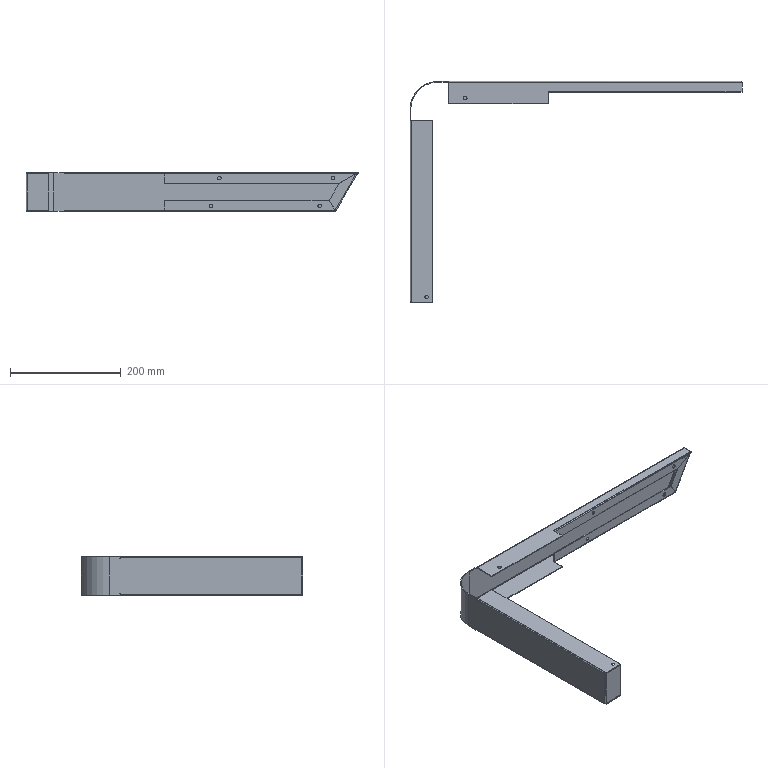Part | SolidWorks | features MirrorStock 1 | 1 solid | 128 faces | box 600.7 x 400 x 70 mm | volume 200425 mm3 | plane 87 | cylinder 36 | spline 5 | commonest cylinder face diameters 6.4 x16 1 x9 4 x9 97 x1 100 x1